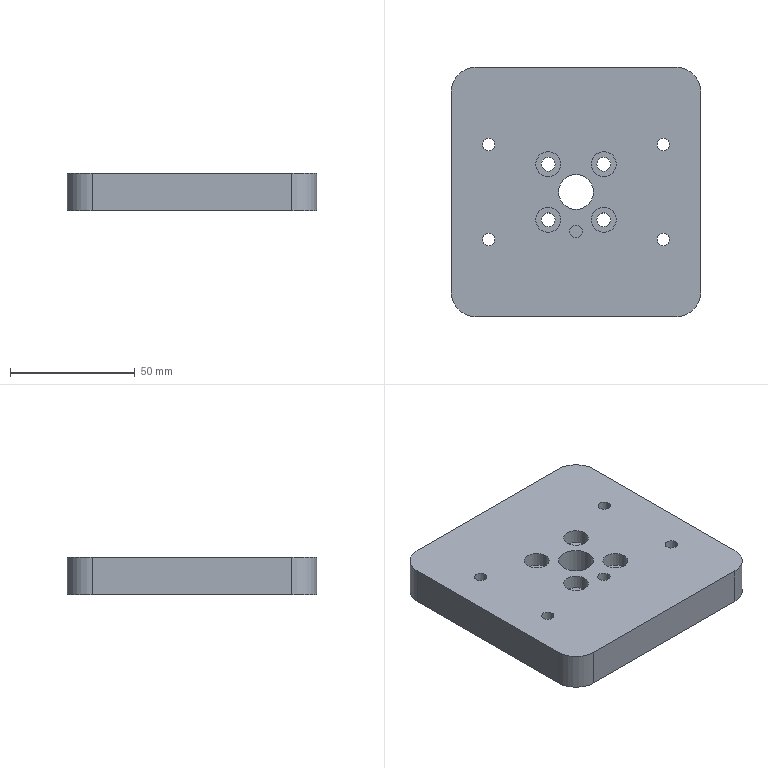NC program | NX | posted with a generic post | part box 100 x 100 x 15 mm
Lines 1755 to 2072 of 2072:
(DRILLING , TOOL : D6A45)
N3484 T07 M6
N3486 G54
N3488 G17 G0 G90 X35. Y19. S5000 M3
N3490 G43 Z30. H7
N3492 G94 G81 G98 Z-1. F250. R3.
N3494 X11.137 Y11.137
N3496 X0. Y0.
N3498 X-11.137 Y11.137
N3500 X-35. Y19.
N3502 Y-19.
N3504 X-11.137 Y-11.137
N3506 X0. Y-15.75
N3508 X11.137 Y-11.137
N3510 X35. Y-19.
N3512 G80
N3514 G0 X35. Y-19. Z30.
N3516 M5
(DRILLING_COPY , TOOL : 5.0ZT)
N3518 T15 M6
N3520 G54
N3522 G17 G0 G90 X-35. Y-19. S2000 M3
N3524 G43 Z30. H15
N3526 G94 G83 G98 Z-18.002 F250. Q2. R3.
N3528 Y19.
N3530 X35.
N3532 Y-19.
N3534 G80
N3536 G0 X35. Y-19. Z30.
N3538 M5
(DRILLING_COPY_COPY , TOOL : 5.5ZT)
N3540 T16 M6
N3542 G54
N3544 G17 G0 G90 X-11.137 Y-11.137 S2000 M3
N3546 G43 Z30. H16
N3548 G94 G83 G98 Z-16.652 F250. Q2. R3.
N3550 Y11.137
N3552 X11.137
N3554 Y-11.137
N3556 G80
N3558 G0 X11.137 Y-11.137 Z30.
N3560 M5
(HOLE_MILLING_1 , TOOL : D6)
N3562 T06 M6
N3564 G54
N3566 G17 G0 G90 X-11.137 Y-11.137 S9500 M3
N3568 G43 Z30. H6
N3570 Z0.5
N3572 G94 G3 X-10.137 Y-12.137 R1. F1500.
N3574 X-9.137 Y-11.137 R1.
N3576 X-9.137 Y-11.137 Z0. I-2. J0.
N3578 X-9.137 Y-11.137 Z-0.5 I-2. J0.
N3580 X-9.137 Y-11.137 Z-1. I-2. J0.
N3582 X-9.137 Y-11.137 Z-1.5 I-2. J0.
N3584 X-9.137 Y-11.137 Z-2. I-2. J0.
N3586 X-9.137 Y-11.137 Z-2.5 I-2. J0.
N3588 X-9.137 Y-11.137 Z-3. I-2. J0.
N3590 X-9.137 Y-11.137 Z-3.5 I-2. J0.
N3592 X-9.137 Y-11.137 Z-4. I-2. J0.
N3594 X-9.137 Y-11.137 Z-4.5 I-2. J0.
N3596 X-9.137 Y-11.137 Z-5. I-2. J0.
N3598 X-9.137 Y-11.137 Z-5.5 I-2. J0.
N3600 X-12.755 Y-9.961 Z-5.7 R2.
N3602 X-12.313 Y-12.755 R2.
N3604 X-12.755 Y-9.961 R-2.
N3606 X-12.534 Y-11.358 R1.
N3608 X-11.137 Y-11.137 R1.
N3610 G0 Z30.
N3612 Y11.137
N3614 Z0.5
N3616 G3 X-10.137 Y10.137 R1.
N3618 X-9.137 Y11.137 R1.
N3620 X-9.137 Y11.137 Z0. I-2. J0.
N3622 X-9.137 Y11.137 Z-0.5 I-2. J0.
N3624 X-9.137 Y11.137 Z-1. I-2. J0.
N3626 X-9.137 Y11.137 Z-1.5 I-2. J0.
N3628 X-9.137 Y11.137 Z-2. I-2. J0.
N3630 X-9.137 Y11.137 Z-2.5 I-2. J0.
N3632 X-9.137 Y11.137 Z-3. I-2. J0.
N3634 X-9.137 Y11.137 Z-3.5 I-2. J0.
N3636 X-9.137 Y11.137 Z-4. I-2. J0.
N3638 X-9.137 Y11.137 Z-4.5 I-2. J0.
N3640 X-9.137 Y11.137 Z-5. I-2. J0.
N3642 X-9.137 Y11.137 Z-5.5 I-2. J0.
N3644 X-12.755 Y12.313 Z-5.7 R2.
N3646 X-12.313 Y9.519 R2.
N3648 X-12.755 Y12.313 R-2.
N3650 X-12.534 Y10.916 R1.
N3652 X-11.137 Y11.137 R1.
N3654 G0 Z30.
N3656 X11.137
N3658 Z0.5
N3660 G3 X12.137 Y10.137 R1.
N3662 X13.137 Y11.137 R1.
N3664 X13.137 Y11.137 Z0. I-2. J0.
N3666 X13.137 Y11.137 Z-0.5 I-2. J0.
N3668 X13.137 Y11.137 Z-1. I-2. J0.
N3670 X13.137 Y11.137 Z-1.5 I-2. J0.
N3672 X13.137 Y11.137 Z-2. I-2. J0.
N3674 X13.137 Y11.137 Z-2.5 I-2. J0.
N3676 X13.137 Y11.137 Z-3. I-2. J0.
N3678 X13.137 Y11.137 Z-3.5 I-2. J0.
N3680 X13.137 Y11.137 Z-4. I-2. J0.
N3682 X13.137 Y11.137 Z-4.5 I-2. J0.
N3684 X13.137 Y11.137 Z-5. I-2. J0.
N3686 X13.137 Y11.137 Z-5.5 I-2. J0.
N3688 X9.519 Y12.313 Z-5.7 R2.
N3690 X9.961 Y9.519 R2.
N3692 X9.519 Y12.313 R-2.
N3694 X9.74 Y10.916 R1.
N3696 X11.137 Y11.137 R1.
N3698 G0 Z30.
N3700 Y-11.137
N3702 Z0.5
N3704 G3 X12.137 Y-12.137 R1.
N3706 X13.137 Y-11.137 R1.
N3708 X13.137 Y-11.137 Z0. I-2. J0.
N3710 X13.137 Y-11.137 Z-0.5 I-2. J0.
N3712 X13.137 Y-11.137 Z-1. I-2. J0.
N3714 X13.137 Y-11.137 Z-1.5 I-2. J0.
N3716 X13.137 Y-11.137 Z-2. I-2. J0.
N3718 X13.137 Y-11.137 Z-2.5 I-2. J0.
N3720 X13.137 Y-11.137 Z-3. I-2. J0.
N3722 X13.137 Y-11.137 Z-3.5 I-2. J0.
N3724 X13.137 Y-11.137 Z-4. I-2. J0.
N3726 X13.137 Y-11.137 Z-4.5 I-2. J0.
N3728 X13.137 Y-11.137 Z-5. I-2. J0.
N3730 X13.137 Y-11.137 Z-5.5 I-2. J0.
N3732 X9.519 Y-9.961 Z-5.7 R2.
N3734 X9.961 Y-12.755 R2.
N3736 X9.519 Y-9.961 R-2.
N3738 X9.74 Y-11.358 R1.
N3740 X11.137 Y-11.137 R1.
N3742 G0 Z30.
N3744 M5
(HOLE_MILLING_1_COPY , TOOL : D3)
N3746 T03 M6
N3748 G54
N3750 G17 G0 G90 X0. Y-15.75 S9500 M3
N3752 G43 Z30. H3
N3754 Z0.5
N3756 G94 G3 X0.45 Y-16.2 R0.45 F1000.
N3758 X0.9 Y-15.75 R0.45
N3760 X0.9 Y-15.75 Z0.2 I-0.9 J0.
N3762 X0.9 Y-15.75 Z-0.1 I-0.9 J0.
N3764 X0.9 Y-15.75 Z-0.4 I-0.9 J0.
N3766 X0.9 Y-15.75 Z-0.7 I-0.9 J0.
N3768 X0.9 Y-15.75 Z-1. I-0.9 J0.
N3770 X0.9 Y-15.75 Z-1.3 I-0.9 J0.
N3772 X0.9 Y-15.75 Z-1.6 I-0.9 J0.
N3774 X0.9 Y-15.75 Z-1.9 I-0.9 J0.
N3776 X0.9 Y-15.75 Z-2.2 I-0.9 J0.
N3778 X0.9 Y-15.75 Z-2.5 I-0.9 J0.
N3780 X0.9 Y-15.75 Z-2.8 I-0.9 J0.
N3782 X0.9 Y-15.75 Z-3.1 I-0.9 J0.
N3784 X0.9 Y-15.75 Z-3.4 I-0.9 J0.
N3786 X0.9 Y-15.75 Z-3.7 I-0.9 J0.
N3788 X0.9 Y-15.75 Z-4. I-0.9 J0.
N3790 X0.9 Y-15.75 Z-4.3 I-0.9 J0.
N3792 X0.9 Y-15.75 Z-4.6 I-0.9 J0.
N3794 X0.9 Y-15.75 Z-4.9 I-0.9 J0.
N3796 X0.9 Y-15.75 Z-5.2 I-0.9 J0.
N3798 X0.9 Y-15.75 Z-5.5 I-0.9 J0.
N3800 X0.9 Y-15.75 Z-5.8 I-0.9 J0.
N3802 X0.9 Y-15.75 Z-6.1 I-0.9 J0.
N3804 X0.9 Y-15.75 Z-6.4 I-0.9 J0.
N3806 X-0.45 Y-14.971 Z-6.5 R0.9
N3808 X-0.779 Y-16.2 R0.9
N3810 X-0.45 Y-14.971 R-0.9
N3812 X-0.615 Y-15.585 R0.45
N3814 X0. Y-15.75 R0.45
N3816 G0 Z30.
N3818 M5
(PLANAR_MILL , TOOL : D6A45)
N3820 T07 M6
N3822 G54
N3824 G17 G0 G90 X36.1 Y-19.866 S9500 M3
N3826 G43 Z30. H7
N3828 Z0.5
N3830 G94 G1 Z-1. F1250.
N3832 G3 X36.6 Y-19. R1.
N3834 X35. Y-17.4 R1.6
N3836 X36.6 Y-19. R-1.6
N3838 X36.1 Y-18.134 R1.
N3840 G1 Z0.5
N3842 G0 Z30.
N3844 X14.737 Y-12.003
N3846 Z0.5
N3848 G1 Z-1.
N3850 G3 X15.237 Y-11.137 R1.
N3852 X11.137 Y-7.037 R4.1
N3854 X15.237 Y-11.137 R-4.1
N3856 X14.737 Y-10.271 R1.
N3858 G1 Z0.5
N3860 G0 Z30.
N3862 X-0.866 Y-16.85
N3864 Z0.5
N3866 G1 Z-1.
N3868 G3 X0. Y-17.35 R1.
N3870 X1.6 Y-15.75 R1.6
N3872 X0. Y-17.35 R-1.6
N3874 X0.866 Y-16.85 R1.
N3876 G1 Z0.5
N3878 G0 Z30.
N3880 X-12.003 Y-14.737
N3882 Z0.5
N3884 G1 Z-1.
N3886 G3 X-11.137 Y-15.237 R1.
N3888 X-7.037 Y-11.137 R4.1
N3890 X-11.137 Y-15.237 R-4.1
N3892 X-10.271 Y-14.737 R1.
N3894 G1 Z0.5
N3896 G0 Z30.
N3898 X-36.1 Y-18.134
N3900 Z0.5
N3902 G1 Z-1.
N3904 G3 X-36.6 Y-19. R1.
N3906 X-35. Y-20.6 R1.6
N3908 X-36.6 Y-19. R-1.6
N3910 X-36.1 Y-19.866 R1.
N3912 G1 Z0.5
N3914 G0 Z30.
N3916 Y19.866
N3918 Z0.5
N3920 G1 Z-1.
N3922 G3 X-36.6 Y19. R1.
N3924 X-35. Y17.4 R1.6
N3926 X-36.6 Y19. R-1.6
N3928 X-36.1 Y18.134 R1.
N3930 G1 Z0.5
N3932 G0 Z30.
N3934 X-14.737 Y12.003
N3936 Z0.5
N3938 G1 Z-1.
N3940 G3 X-15.237 Y11.137 R1.
N3942 X-11.137 Y7.037 R4.1
N3944 X-15.237 Y11.137 R-4.1
N3946 X-14.737 Y10.271 R1.
N3948 G1 Z0.5
N3950 G0 Z30.
N3952 X-51.4 Y-0.866
N3954 Z0.5
N3956 G1 Z-1.
N3958 G3 X-50.9 Y0. R1.
N3960 G1 Y40.
N3962 G2 X-40. Y50.9 R10.9
N3964 G1 X40.
N3966 G2 X50.9 Y40. R10.9
N3968 G1 Y-40.
N3970 G2 X40. Y-50.9 R10.9
N3972 G1 X-40.
N3974 G2 X-50.9 Y-40. R10.9
N3976 G1 Y0.
N3978 G3 X-51.4 Y0.866 R1.
N3980 G1 Z0.5
N3982 G0 Z30.
N3984 X-5.6
N3986 Z0.5
N3988 G1 Z-1.
N3990 G3 X-6.1 Y0. R1.
N3992 X0. Y-6.1 R6.1
N3994 X-6.1 Y0. R-6.1
N3996 X-5.6 Y-0.866 R1.
N3998 G1 Z0.5
N4000 G0 Z30.
N4002 X14.737 Y10.271
N4004 Z0.5
N4006 G1 Z-1.
N4008 G3 X15.237 Y11.137 R1.
N4010 X11.137 Y15.237 R4.1
N4012 X15.237 Y11.137 R-4.1
N4014 X14.737 Y12.003 R1.
N4016 G1 Z0.5
N4018 G0 Z30.
N4020 X36.1 Y18.134
N4022 Z0.5
N4024 G1 Z-1.
N4026 G3 X36.6 Y19. R1.
N4028 X35. Y20.6 R1.6
N4030 X36.6 Y19. R-1.6
N4032 X36.1 Y19.866 R1.
N4034 G1 Z0.5
N4036 G0 Z30.
N4038 M5
(刀补3 , TOOL : D3)
N4040 T03 M6
N4042 G54
N4044 G17 G0 G90 X0. Y-15.75 S9500 M3
N4046 G43 Z30. H3
N4048 Z0.5
N4050 G41 G94 G1 X0.004 Y-15.85 F1000. D3
N4052 G3 X0.95 Y-15.75 R0.478
N4054 X0.95 Y-15.75 Z-1.5 I-0.95 J0.
N4056 X0.95 Y-15.75 Z-3.5 I-0.95 J0.
N4058 X0.95 Y-15.75 Z-5.5 I-0.95 J0.
N4060 X-0.95 Y-15.75 Z-6.5 I-0.95 J0.
N4062 X0. Y-16.7 R0.95
N4064 X-0.95 Y-15.75 R-0.95
N4066 X-0.004 Y-15.85 R0.478
N4068 G40
N4070 G1 X0. Y-15.75
N4072 G0 Z30.
N4074 M5
N4076 M2